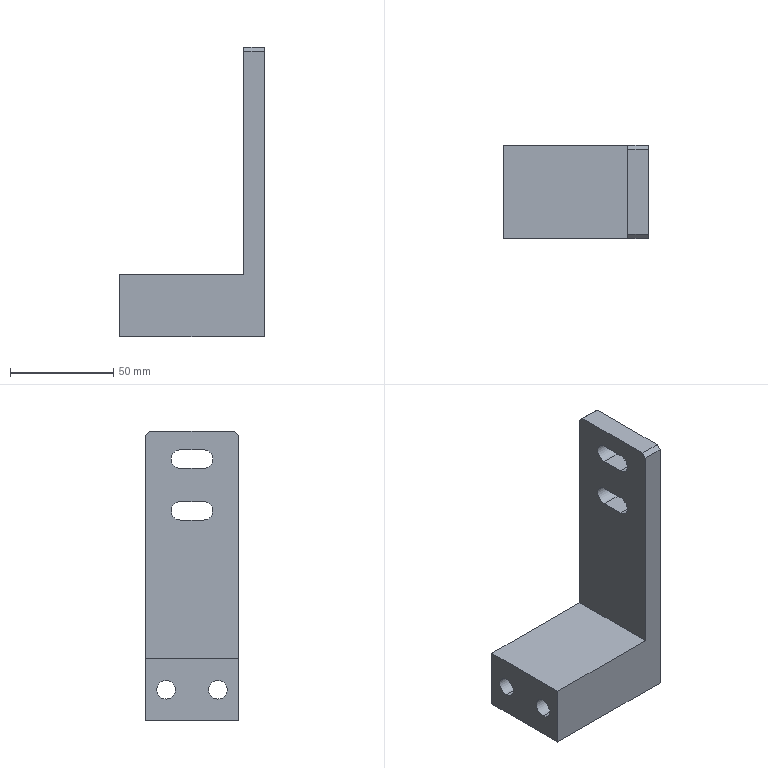Part | SolidWorks | features BaseBody 1 | 1 solid | 28 faces | box 70 x 45 x 140 mm | volume 118230 mm3 | plane 16 | cylinder 12 | commonest cylinder face diameters 9 x8 15 x4
STEP:
#1=CARTESIAN_POINT('',(114.247,1537.,-339.5));
#2=VERTEX_POINT('',#1);
#3=CARTESIAN_POINT('',(114.247,1537.,-354.5));
#4=VERTEX_POINT('',#3);
#5=CARTESIAN_POINT('',(114.247,1537.,-347.));
#6=DIRECTION('',(1.,0.,0.));
#7=DIRECTION('',(0.,0.,-1.));
#8=AXIS2_PLACEMENT_3D('',#5,#6,#7);
#9=CIRCLE('',#8,7.5);
#10=EDGE_CURVE('',#2,#4,#9,.T.);
#11=ORIENTED_EDGE('',*,*,#10,.F.);
#12=CARTESIAN_POINT('',(174.247,1537.,-339.5));
#13=VERTEX_POINT('',#12);
#14=CARTESIAN_POINT('',(174.247,1537.,-339.5));
#15=DIRECTION('',(1.,0.,0.));
#16=VECTOR('',#15,1000.);
#17=LINE('',#14,#16);
#18=EDGE_CURVE('',#2,#13,#17,.T.);
#19=ORIENTED_EDGE('',*,*,#18,.T.);
#20=CARTESIAN_POINT('',(174.247,1537.,-354.5));
#21=VERTEX_POINT('',#20);
#22=CARTESIAN_POINT('',(174.247,1537.,-347.));
#23=DIRECTION('',(1.,0.,0.));
#24=DIRECTION('',(0.,0.,-1.));
#25=AXIS2_PLACEMENT_3D('',#22,#23,#24);
#26=CIRCLE('',#25,7.5);
#27=EDGE_CURVE('',#13,#21,#26,.T.);
#28=ORIENTED_EDGE('',*,*,#27,.T.);
#29=CARTESIAN_POINT('',(174.247,1537.,-354.5));
#30=DIRECTION('',(1.,0.,0.));
#31=VECTOR('',#30,1000.);
#32=LINE('',#29,#31);
#33=EDGE_CURVE('',#4,#21,#32,.T.);
#34=ORIENTED_EDGE('',*,*,#33,.F.);
#35=EDGE_LOOP('',(#11,#19,#28,#34));
#36=FACE_OUTER_BOUND('',#35,.T.);
#37=CARTESIAN_POINT('',(174.247,1537.,-347.));
#38=DIRECTION('',(1.,0.,0.));
#39=DIRECTION('',(0.,0.,-1.));
#40=AXIS2_PLACEMENT_3D('',#37,#38,#39);
#41=CYLINDRICAL_SURFACE('',#40,7.5);
#42=ADVANCED_FACE('',(#36),#41,.F.);
#43=CARTESIAN_POINT('',(114.247,1562.,-339.5));
#44=VERTEX_POINT('',#43);
#45=CARTESIAN_POINT('',(114.247,1562.,-354.5));
#46=VERTEX_POINT('',#45);
#47=CARTESIAN_POINT('',(114.247,1562.,-347.));
#48=DIRECTION('',(1.,0.,0.));
#49=DIRECTION('',(0.,0.,-1.));
#50=AXIS2_PLACEMENT_3D('',#47,#48,#49);
#51=CIRCLE('',#50,7.5);
#52=EDGE_CURVE('',#44,#46,#51,.T.);
#53=ORIENTED_EDGE('',*,*,#52,.F.);
#54=CARTESIAN_POINT('',(174.247,1562.,-339.5));
#55=VERTEX_POINT('',#54);
#56=CARTESIAN_POINT('',(174.247,1562.,-339.5));
#57=DIRECTION('',(1.,0.,0.));
#58=VECTOR('',#57,1000.);
#59=LINE('',#56,#58);
#60=EDGE_CURVE('',#44,#55,#59,.T.);
#61=ORIENTED_EDGE('',*,*,#60,.T.);
#62=CARTESIAN_POINT('',(174.247,1562.,-354.5));
#63=VERTEX_POINT('',#62);
#64=CARTESIAN_POINT('',(174.247,1562.,-347.));
#65=DIRECTION('',(1.,0.,0.));
#66=DIRECTION('',(0.,0.,-1.));
#67=AXIS2_PLACEMENT_3D('',#64,#65,#66);
#68=CIRCLE('',#67,7.5);
#69=EDGE_CURVE('',#55,#63,#68,.T.);
#70=ORIENTED_EDGE('',*,*,#69,.T.);
#71=CARTESIAN_POINT('',(174.247,1562.,-354.5));
#72=DIRECTION('',(1.,0.,0.));
#73=VECTOR('',#72,1000.);
#74=LINE('',#71,#73);
#75=EDGE_CURVE('',#46,#63,#74,.T.);
#76=ORIENTED_EDGE('',*,*,#75,.F.);
#77=EDGE_LOOP('',(#53,#61,#70,#76));
#78=FACE_OUTER_BOUND('',#77,.T.);
#79=CARTESIAN_POINT('',(174.247,1562.,-347.));
#80=DIRECTION('',(1.,0.,0.));
#81=DIRECTION('',(0.,0.,-1.));
#82=AXIS2_PLACEMENT_3D('',#79,#80,#81);
#83=CYLINDRICAL_SURFACE('',#82,7.5);
#84=ADVANCED_FACE('',(#78),#83,.F.);
#85=CARTESIAN_POINT('',(104.247,1537.,-351.5));
#86=VERTEX_POINT('',#85);
#87=CARTESIAN_POINT('',(104.247,1537.,-342.5));
#88=VERTEX_POINT('',#87);
#89=CARTESIAN_POINT('',(104.247,1537.,-347.));
#90=DIRECTION('',(-1.,0.,0.));
#91=DIRECTION('',(0.,0.,-1.));
#92=AXIS2_PLACEMENT_3D('',#89,#90,#91);
#93=CIRCLE('',#92,4.5);
#94=EDGE_CURVE('',#86,#88,#93,.T.);
#95=ORIENTED_EDGE('',*,*,#94,.T.);
#96=CARTESIAN_POINT('',(114.247,1537.,-342.5));
#97=VERTEX_POINT('',#96);
#98=CARTESIAN_POINT('',(174.247,1537.,-342.5));
#99=DIRECTION('',(1.,0.,0.));
#100=VECTOR('',#99,1000.);
#101=LINE('',#98,#100);
#102=EDGE_CURVE('',#88,#97,#101,.T.);
#103=ORIENTED_EDGE('',*,*,#102,.T.);
#104=CARTESIAN_POINT('',(114.247,1537.,-351.5));
#105=VERTEX_POINT('',#104);
#106=CARTESIAN_POINT('',(114.247,1537.,-347.));
#107=DIRECTION('',(1.,0.,0.));
#108=DIRECTION('',(0.,0.,-1.));
#109=AXIS2_PLACEMENT_3D('',#106,#107,#108);
#110=CIRCLE('',#109,4.5);
#111=EDGE_CURVE('',#97,#105,#110,.T.);
#112=ORIENTED_EDGE('',*,*,#111,.T.);
#113=CARTESIAN_POINT('',(174.247,1537.,-351.5));
#114=DIRECTION('',(1.,0.,0.));
#115=VECTOR('',#114,1000.);
#116=LINE('',#113,#115);
#117=EDGE_CURVE('',#86,#105,#116,.T.);
#118=ORIENTED_EDGE('',*,*,#117,.F.);
#119=EDGE_LOOP('',(#95,#103,#112,#118));
#120=FACE_OUTER_BOUND('',#119,.T.);
#121=CARTESIAN_POINT('',(174.247,1537.,-347.));
#122=DIRECTION('',(1.,0.,0.));
#123=DIRECTION('',(0.,0.,-1.));
#124=AXIS2_PLACEMENT_3D('',#121,#122,#123);
#125=CYLINDRICAL_SURFACE('',#124,4.5);
#126=ADVANCED_FACE('',(#120),#125,.F.);
#127=CARTESIAN_POINT('',(104.247,1562.,-351.5));
#128=VERTEX_POINT('',#127);
#129=CARTESIAN_POINT('',(104.247,1562.,-342.5));
#130=VERTEX_POINT('',#129);
#131=CARTESIAN_POINT('',(104.247,1562.,-347.));
#132=DIRECTION('',(-1.,0.,0.));
#133=DIRECTION('',(0.,0.,-1.));
#134=AXIS2_PLACEMENT_3D('',#131,#132,#133);
#135=CIRCLE('',#134,4.5);
#136=EDGE_CURVE('',#128,#130,#135,.T.);
#137=ORIENTED_EDGE('',*,*,#136,.T.);
#138=CARTESIAN_POINT('',(114.247,1562.,-342.5));
#139=VERTEX_POINT('',#138);
#140=CARTESIAN_POINT('',(174.247,1562.,-342.5));
#141=DIRECTION('',(1.,0.,0.));
#142=VECTOR('',#141,1000.);
#143=LINE('',#140,#142);
#144=EDGE_CURVE('',#130,#139,#143,.T.);
#145=ORIENTED_EDGE('',*,*,#144,.T.);
#146=CARTESIAN_POINT('',(114.247,1562.,-351.5));
#147=VERTEX_POINT('',#146);
#148=CARTESIAN_POINT('',(114.247,1562.,-347.));
#149=DIRECTION('',(1.,0.,0.));
#150=DIRECTION('',(0.,0.,-1.));
#151=AXIS2_PLACEMENT_3D('',#148,#149,#150);
#152=CIRCLE('',#151,4.5);
#153=EDGE_CURVE('',#139,#147,#152,.T.);
#154=ORIENTED_EDGE('',*,*,#153,.T.);
#155=CARTESIAN_POINT('',(174.247,1562.,-351.5));
#156=DIRECTION('',(1.,0.,0.));
#157=VECTOR('',#156,1000.);
#158=LINE('',#155,#157);
#159=EDGE_CURVE('',#128,#147,#158,.T.);
#160=ORIENTED_EDGE('',*,*,#159,.F.);
#161=EDGE_LOOP('',(#137,#145,#154,#160));
#162=FACE_OUTER_BOUND('',#161,.T.);
#163=CARTESIAN_POINT('',(174.247,1562.,-347.));
#164=DIRECTION('',(1.,0.,0.));
#165=DIRECTION('',(0.,0.,-1.));
#166=AXIS2_PLACEMENT_3D('',#163,#164,#165);
#167=CYLINDRICAL_SURFACE('',#166,4.5);
#168=ADVANCED_FACE('',(#162),#167,.F.);
#169=CARTESIAN_POINT('',(174.247,1544.,-240.));
#170=VERTEX_POINT('',#169);
#171=CARTESIAN_POINT('',(174.247,1555.,-240.));
#172=VERTEX_POINT('',#171);
#173=CARTESIAN_POINT('',(174.247,1549.5,-240.));
#174=DIRECTION('',(0.,1.,0.));
#175=VECTOR('',#174,1000.);
#176=LINE('',#173,#175);
#177=EDGE_CURVE('',#170,#172,#176,.T.);
#178=ORIENTED_EDGE('',*,*,#177,.F.);
#179=CARTESIAN_POINT('',(174.247,1544.,-231.));
#180=VERTEX_POINT('',#179);
#181=CARTESIAN_POINT('',(174.247,1544.,-235.5));
#182=DIRECTION('',(1.,0.,0.));
#183=DIRECTION('',(0.,0.,-1.));
#184=AXIS2_PLACEMENT_3D('',#181,#182,#183);
#185=CIRCLE('',#184,4.5);
#186=EDGE_CURVE('',#180,#170,#185,.T.);
#187=ORIENTED_EDGE('',*,*,#186,.F.);
#188=CARTESIAN_POINT('',(174.247,1555.,-231.));
#189=VERTEX_POINT('',#188);
#190=CARTESIAN_POINT('',(174.247,1549.5,-231.));
#191=DIRECTION('',(0.,-1.,0.));
#192=VECTOR('',#191,1000.);
#193=LINE('',#190,#192);
#194=EDGE_CURVE('',#189,#180,#193,.T.);
#195=ORIENTED_EDGE('',*,*,#194,.F.);
#196=CARTESIAN_POINT('',(174.247,1555.,-235.5));
#197=DIRECTION('',(1.,0.,0.));
#198=DIRECTION('',(0.,0.,-1.));
#199=AXIS2_PLACEMENT_3D('',#196,#197,#198);
#200=CIRCLE('',#199,4.5);
#201=EDGE_CURVE('',#172,#189,#200,.T.);
#202=ORIENTED_EDGE('',*,*,#201,.F.);
#203=EDGE_LOOP('',(#178,#187,#195,#202));
#204=FACE_BOUND('',#203,.T.);
#205=CARTESIAN_POINT('',(174.247,1555.,-256.));
#206=VERTEX_POINT('',#205);
#207=CARTESIAN_POINT('',(174.247,1544.,-256.));
#208=VERTEX_POINT('',#207);
#209=CARTESIAN_POINT('',(174.247,1549.5,-256.));
#210=DIRECTION('',(0.,-1.,0.));
#211=VECTOR('',#210,1000.);
#212=LINE('',#209,#211);
#213=EDGE_CURVE('',#206,#208,#212,.T.);
#214=ORIENTED_EDGE('',*,*,#213,.F.);
#215=CARTESIAN_POINT('',(174.247,1555.,-265.));
#216=VERTEX_POINT('',#215);
#217=CARTESIAN_POINT('',(174.247,1555.,-260.5));
#218=DIRECTION('',(1.,0.,0.));
#219=DIRECTION('',(0.,0.,-1.));
#220=AXIS2_PLACEMENT_3D('',#217,#218,#219);
#221=CIRCLE('',#220,4.5);
#222=EDGE_CURVE('',#216,#206,#221,.T.);
#223=ORIENTED_EDGE('',*,*,#222,.F.);
#224=CARTESIAN_POINT('',(174.247,1544.,-265.));
#225=VERTEX_POINT('',#224);
#226=CARTESIAN_POINT('',(174.247,1549.5,-265.));
#227=DIRECTION('',(0.,1.,0.));
#228=VECTOR('',#227,1000.);
#229=LINE('',#226,#228);
#230=EDGE_CURVE('',#225,#216,#229,.T.);
#231=ORIENTED_EDGE('',*,*,#230,.F.);
#232=CARTESIAN_POINT('',(174.247,1544.,-260.5));
#233=DIRECTION('',(1.,0.,0.));
#234=DIRECTION('',(0.,0.,-1.));
#235=AXIS2_PLACEMENT_3D('',#232,#233,#234);
#236=CIRCLE('',#235,4.5);
#237=EDGE_CURVE('',#208,#225,#236,.T.);
#238=ORIENTED_EDGE('',*,*,#237,.F.);
#239=EDGE_LOOP('',(#214,#223,#231,#238));
#240=FACE_BOUND('',#239,.T.);
#241=CARTESIAN_POINT('',(174.247,1537.,-347.));
#242=DIRECTION('',(1.,0.,0.));
#243=DIRECTION('',(0.,0.,-1.));
#244=AXIS2_PLACEMENT_3D('',#241,#242,#243);
#245=CIRCLE('',#244,7.5);
#246=EDGE_CURVE('',#21,#13,#245,.T.);
#247=ORIENTED_EDGE('',*,*,#246,.F.);
#248=ORIENTED_EDGE('',*,*,#27,.F.);
#249=EDGE_LOOP('',(#247,#248));
#250=FACE_BOUND('',#249,.T.);
#251=CARTESIAN_POINT('',(174.247,1562.,-347.));
#252=DIRECTION('',(1.,0.,0.));
#253=DIRECTION('',(0.,0.,-1.));
#254=AXIS2_PLACEMENT_3D('',#251,#252,#253);
#255=CIRCLE('',#254,7.5);
#256=EDGE_CURVE('',#63,#55,#255,.T.);
#257=ORIENTED_EDGE('',*,*,#256,.F.);
#258=ORIENTED_EDGE('',*,*,#69,.F.);
#259=EDGE_LOOP('',(#257,#258));
#260=FACE_BOUND('',#259,.T.);
#261=CARTESIAN_POINT('',(174.247,1529.,-222.));
#262=VERTEX_POINT('',#261);
#263=CARTESIAN_POINT('',(174.247,1570.,-222.));
#264=VERTEX_POINT('',#263);
#265=CARTESIAN_POINT('',(174.247,1549.5,-222.));
#266=DIRECTION('',(0.,1.,0.));
#267=VECTOR('',#266,1000.);
#268=LINE('',#265,#267);
#269=EDGE_CURVE('',#262,#264,#268,.T.);
#270=ORIENTED_EDGE('',*,*,#269,.F.);
#271=CARTESIAN_POINT('',(174.247,1527.,-224.));
#272=VERTEX_POINT('',#271);
#273=CARTESIAN_POINT('',(174.247,1527.,-224.));
#274=DIRECTION('',(0.,0.7071,0.7071));
#275=VECTOR('',#274,1000.);
#276=LINE('',#273,#275);
#277=EDGE_CURVE('',#272,#262,#276,.T.);
#278=ORIENTED_EDGE('',*,*,#277,.F.);
#279=CARTESIAN_POINT('',(174.247,1527.,-362.));
#280=VERTEX_POINT('',#279);
#281=CARTESIAN_POINT('',(174.247,1527.,-292.));
#282=DIRECTION('',(0.,0.,1.));
#283=VECTOR('',#282,1000.);
#284=LINE('',#281,#283);
#285=EDGE_CURVE('',#280,#272,#284,.T.);
#286=ORIENTED_EDGE('',*,*,#285,.F.);
#287=CARTESIAN_POINT('',(174.247,1572.,-362.));
#288=VERTEX_POINT('',#287);
#289=CARTESIAN_POINT('',(174.247,1549.5,-362.));
#290=DIRECTION('',(0.,-1.,0.));
#291=VECTOR('',#290,1000.);
#292=LINE('',#289,#291);
#293=EDGE_CURVE('',#288,#280,#292,.T.);
#294=ORIENTED_EDGE('',*,*,#293,.F.);
#295=CARTESIAN_POINT('',(174.247,1572.,-224.));
#296=VERTEX_POINT('',#295);
#297=CARTESIAN_POINT('',(174.247,1572.,-292.));
#298=DIRECTION('',(0.,0.,-1.));
#299=VECTOR('',#298,1000.);
#300=LINE('',#297,#299);
#301=EDGE_CURVE('',#296,#288,#300,.T.);
#302=ORIENTED_EDGE('',*,*,#301,.F.);
#303=CARTESIAN_POINT('',(174.247,1570.,-222.));
#304=DIRECTION('',(0.,0.7071,-0.7071));
#305=VECTOR('',#304,1000.);
#306=LINE('',#303,#305);
#307=EDGE_CURVE('',#264,#296,#306,.T.);
#308=ORIENTED_EDGE('',*,*,#307,.F.);
#309=EDGE_LOOP('',(#270,#278,#286,#294,#302,#308));
#310=FACE_OUTER_BOUND('',#309,.T.);
#311=CARTESIAN_POINT('',(174.247,1549.5,-292.));
#312=DIRECTION('',(-1.,0.,0.));
#313=DIRECTION('',(0.,0.,1.));
#314=AXIS2_PLACEMENT_3D('',#311,#312,#313);
#315=PLANE('',#314);
#316=ADVANCED_FACE('',(#204,#240,#250,#260,#310),#315,.F.);
#317=ORIENTED_EDGE('',*,*,#177,.T.);
#318=CARTESIAN_POINT('',(164.247,1555.,-240.));
#319=VERTEX_POINT('',#318);
#320=CARTESIAN_POINT('',(174.247,1555.,-240.));
#321=DIRECTION('',(1.,0.,0.));
#322=VECTOR('',#321,1000.);
#323=LINE('',#320,#322);
#324=EDGE_CURVE('',#319,#172,#323,.T.);
#325=ORIENTED_EDGE('',*,*,#324,.F.);
#326=CARTESIAN_POINT('',(164.247,1544.,-240.));
#327=VERTEX_POINT('',#326);
#328=CARTESIAN_POINT('',(164.247,1544.,-240.));
#329=DIRECTION('',(0.,1.,0.));
#330=VECTOR('',#329,1000.);
#331=LINE('',#328,#330);
#332=EDGE_CURVE('',#327,#319,#331,.T.);
#333=ORIENTED_EDGE('',*,*,#332,.F.);
#334=CARTESIAN_POINT('',(174.247,1544.,-240.));
#335=DIRECTION('',(-1.,0.,0.));
#336=VECTOR('',#335,1000.);
#337=LINE('',#334,#336);
#338=EDGE_CURVE('',#170,#327,#337,.T.);
#339=ORIENTED_EDGE('',*,*,#338,.F.);
#340=EDGE_LOOP('',(#317,#325,#333,#339));
#341=FACE_OUTER_BOUND('',#340,.T.);
#342=CARTESIAN_POINT('',(174.247,1544.,-240.));
#343=DIRECTION('',(0.,0.,-1.));
#344=DIRECTION('',(-1.,0.,0.));
#345=AXIS2_PLACEMENT_3D('',#342,#343,#344);
#346=PLANE('',#345);
#347=ADVANCED_FACE('',(#341),#346,.F.);
#348=ORIENTED_EDGE('',*,*,#186,.T.);
#349=ORIENTED_EDGE('',*,*,#338,.T.);
#350=CARTESIAN_POINT('',(164.247,1544.,-231.));
#351=VERTEX_POINT('',#350);
#352=CARTESIAN_POINT('',(164.247,1544.,-235.5));
#353=DIRECTION('',(1.,0.,0.));
#354=DIRECTION('',(0.,0.,-1.));
#355=AXIS2_PLACEMENT_3D('',#352,#353,#354);
#356=CIRCLE('',#355,4.5);
#357=EDGE_CURVE('',#351,#327,#356,.T.);
#358=ORIENTED_EDGE('',*,*,#357,.F.);
#359=CARTESIAN_POINT('',(174.247,1544.,-231.));
#360=DIRECTION('',(-1.,0.,0.));
#361=VECTOR('',#360,1000.);
#362=LINE('',#359,#361);
#363=EDGE_CURVE('',#180,#351,#362,.T.);
#364=ORIENTED_EDGE('',*,*,#363,.F.);
#365=EDGE_LOOP('',(#348,#349,#358,#364));
#366=FACE_OUTER_BOUND('',#365,.T.);
#367=CARTESIAN_POINT('',(174.247,1544.,-235.5));
#368=DIRECTION('',(1.,0.,0.));
#369=DIRECTION('',(0.,0.,-1.));
#370=AXIS2_PLACEMENT_3D('',#367,#368,#369);
#371=CYLINDRICAL_SURFACE('',#370,4.5);
#372=ADVANCED_FACE('',(#366),#371,.F.);
#373=CARTESIAN_POINT('',(164.247,1555.,-231.));
#374=VERTEX_POINT('',#373);
#375=CARTESIAN_POINT('',(164.247,1544.,-231.));
#376=DIRECTION('',(0.,1.,0.));
#377=VECTOR('',#376,1000.);
#378=LINE('',#375,#377);
#379=EDGE_CURVE('',#351,#374,#378,.T.);
#380=ORIENTED_EDGE('',*,*,#379,.T.);
#381=CARTESIAN_POINT('',(104.247,1555.,-231.));
#382=DIRECTION('',(1.,0.,0.));
#383=VECTOR('',#382,1000.);
#384=LINE('',#381,#383);
#385=EDGE_CURVE('',#374,#189,#384,.T.);
#386=ORIENTED_EDGE('',*,*,#385,.T.);
#387=ORIENTED_EDGE('',*,*,#194,.T.);
#388=ORIENTED_EDGE('',*,*,#363,.T.);
#389=EDGE_LOOP('',(#380,#386,#387,#388));
#390=FACE_OUTER_BOUND('',#389,.T.);
#391=CARTESIAN_POINT('',(104.247,1544.,-231.));
#392=DIRECTION('',(0.,0.,-1.));
#393=DIRECTION('',(-1.,0.,0.));
#394=AXIS2_PLACEMENT_3D('',#391,#392,#393);
#395=PLANE('',#394);
#396=ADVANCED_FACE('',(#390),#395,.T.);
#397=ORIENTED_EDGE('',*,*,#324,.T.);
#398=ORIENTED_EDGE('',*,*,#201,.T.);
#399=ORIENTED_EDGE('',*,*,#385,.F.);
#400=CARTESIAN_POINT('',(164.247,1555.,-235.5));
#401=DIRECTION('',(1.,0.,0.));
#402=DIRECTION('',(0.,0.,-1.));
#403=AXIS2_PLACEMENT_3D('',#400,#401,#402);
#404=CIRCLE('',#403,4.5);
#405=EDGE_CURVE('',#319,#374,#404,.T.);
#406=ORIENTED_EDGE('',*,*,#405,.F.);
#407=EDGE_LOOP('',(#397,#398,#399,#406));
#408=FACE_OUTER_BOUND('',#407,.T.);
#409=CARTESIAN_POINT('',(174.247,1555.,-235.5));
#410=DIRECTION('',(1.,0.,0.));
#411=DIRECTION('',(0.,0.,-1.));
#412=AXIS2_PLACEMENT_3D('',#409,#410,#411);
#413=CYLINDRICAL_SURFACE('',#412,4.5);
#414=ADVANCED_FACE('',(#408),#413,.F.);
#415=CARTESIAN_POINT('',(164.247,1544.,-256.));
#416=VERTEX_POINT('',#415);
#417=CARTESIAN_POINT('',(174.247,1544.,-256.));
#418=DIRECTION('',(-1.,0.,0.));
#419=VECTOR('',#418,1000.);
#420=LINE('',#417,#419);
#421=EDGE_CURVE('',#208,#416,#420,.T.);
#422=ORIENTED_EDGE('',*,*,#421,.F.);
#423=ORIENTED_EDGE('',*,*,#237,.T.);
#424=CARTESIAN_POINT('',(164.247,1544.,-265.));
#425=VERTEX_POINT('',#424);
#426=CARTESIAN_POINT('',(174.247,1544.,-265.));
#427=DIRECTION('',(1.,0.,0.));
#428=VECTOR('',#427,1000.);
#429=LINE('',#426,#428);
#430=EDGE_CURVE('',#425,#225,#429,.T.);
#431=ORIENTED_EDGE('',*,*,#430,.F.);
#432=CARTESIAN_POINT('',(164.247,1544.,-260.5));
#433=DIRECTION('',(1.,0.,0.));
#434=DIRECTION('',(0.,0.,-1.));
#435=AXIS2_PLACEMENT_3D('',#432,#433,#434);
#436=CIRCLE('',#435,4.5);
#437=EDGE_CURVE('',#416,#425,#436,.T.);
#438=ORIENTED_EDGE('',*,*,#437,.F.);
#439=EDGE_LOOP('',(#422,#423,#431,#438));
#440=FACE_OUTER_BOUND('',#439,.T.);
#441=CARTESIAN_POINT('',(174.247,1544.,-260.5));
#442=DIRECTION('',(1.,0.,0.));
#443=DIRECTION('',(0.,0.,-1.));
#444=AXIS2_PLACEMENT_3D('',#441,#442,#443);
#445=CYLINDRICAL_SURFACE('',#444,4.5);
#446=ADVANCED_FACE('',(#440),#445,.F.);
#447=CARTESIAN_POINT('',(164.247,1555.,-256.));
#448=VERTEX_POINT('',#447);
#449=CARTESIAN_POINT('',(164.247,1544.,-256.));
#450=DIRECTION('',(0.,1.,0.));
#451=VECTOR('',#450,1000.);
#452=LINE('',#449,#451);
#453=EDGE_CURVE('',#416,#448,#452,.T.);
#454=ORIENTED_EDGE('',*,*,#453,.T.);
#455=CARTESIAN_POINT('',(104.247,1555.,-256.));
#456=DIRECTION('',(1.,0.,0.));
#457=VECTOR('',#456,1000.);
#458=LINE('',#455,#457);
#459=EDGE_CURVE('',#448,#206,#458,.T.);
#460=ORIENTED_EDGE('',*,*,#459,.T.);
#461=ORIENTED_EDGE('',*,*,#213,.T.);
#462=ORIENTED_EDGE('',*,*,#421,.T.);
#463=EDGE_LOOP('',(#454,#460,#461,#462));
#464=FACE_OUTER_BOUND('',#463,.T.);
#465=CARTESIAN_POINT('',(104.247,1544.,-256.));
#466=DIRECTION('',(0.,0.,-1.));
#467=DIRECTION('',(-1.,0.,0.));
#468=AXIS2_PLACEMENT_3D('',#465,#466,#467);
#469=PLANE('',#468);
#470=ADVANCED_FACE('',(#464),#469,.T.);
#471=CARTESIAN_POINT('',(164.247,1555.,-265.));
#472=VERTEX_POINT('',#471);
#473=CARTESIAN_POINT('',(174.247,1555.,-265.));
#474=DIRECTION('',(-1.,0.,0.));
#475=VECTOR('',#474,1000.);
#476=LINE('',#473,#475);
#477=EDGE_CURVE('',#216,#472,#476,.T.);
#478=ORIENTED_EDGE('',*,*,#477,.F.);
#479=ORIENTED_EDGE('',*,*,#222,.T.);
#480=ORIENTED_EDGE('',*,*,#459,.F.);
#481=CARTESIAN_POINT('',(164.247,1555.,-260.5));
#482=DIRECTION('',(1.,0.,0.));
#483=DIRECTION('',(0.,0.,-1.));
#484=AXIS2_PLACEMENT_3D('',#481,#482,#483);
#485=CIRCLE('',#484,4.5);
#486=EDGE_CURVE('',#472,#448,#485,.T.);
#487=ORIENTED_EDGE('',*,*,#486,.F.);
#488=EDGE_LOOP('',(#478,#479,#480,#487));
#489=FACE_OUTER_BOUND('',#488,.T.);
#490=CARTESIAN_POINT('',(174.247,1555.,-260.5));
#491=DIRECTION('',(1.,0.,0.));
#492=DIRECTION('',(0.,0.,-1.));
#493=AXIS2_PLACEMENT_3D('',#490,#491,#492);
#494=CYLINDRICAL_SURFACE('',#493,4.5);
#495=ADVANCED_FACE('',(#489),#494,.F.);
#496=ORIENTED_EDGE('',*,*,#230,.T.);
#497=ORIENTED_EDGE('',*,*,#477,.T.);
#498=CARTESIAN_POINT('',(164.247,1544.,-265.));
#499=DIRECTION('',(0.,1.,0.));
#500=VECTOR('',#499,1000.);
#501=LINE('',#498,#500);
#502=EDGE_CURVE('',#425,#472,#501,.T.);
#503=ORIENTED_EDGE('',*,*,#502,.F.);
#504=ORIENTED_EDGE('',*,*,#430,.T.);
#505=EDGE_LOOP('',(#496,#497,#503,#504));
#506=FACE_OUTER_BOUND('',#505,.T.);
#507=CARTESIAN_POINT('',(174.247,1544.,-265.));
#508=DIRECTION('',(0.,0.,-1.));
#509=DIRECTION('',(-1.,0.,0.));
#510=AXIS2_PLACEMENT_3D('',#507,#508,#509);
#511=PLANE('',#510);
#512=ADVANCED_FACE('',(#506),#511,.F.);
#513=ORIENTED_EDGE('',*,*,#18,.F.);
#514=CARTESIAN_POINT('',(114.247,1537.,-347.));
#515=DIRECTION('',(1.,0.,0.));
#516=DIRECTION('',(0.,0.,-1.));
#517=AXIS2_PLACEMENT_3D('',#514,#515,#516);
#518=CIRCLE('',#517,7.5);
#519=EDGE_CURVE('',#4,#2,#518,.T.);
#520=ORIENTED_EDGE('',*,*,#519,.F.);
#521=ORIENTED_EDGE('',*,*,#33,.T.);
#522=ORIENTED_EDGE('',*,*,#246,.T.);
#523=EDGE_LOOP('',(#513,#520,#521,#522));
#524=FACE_OUTER_BOUND('',#523,.T.);
#525=CARTESIAN_POINT('',(174.247,1537.,-347.));
#526=DIRECTION('',(1.,0.,0.));
#527=DIRECTION('',(0.,0.,-1.));
#528=AXIS2_PLACEMENT_3D('',#525,#526,#527);
#529=CYLINDRICAL_SURFACE('',#528,7.5);
#530=ADVANCED_FACE('',(#524),#529,.F.);
#531=ORIENTED_EDGE('',*,*,#60,.F.);
#532=CARTESIAN_POINT('',(114.247,1562.,-347.));
#533=DIRECTION('',(1.,0.,0.));
#534=DIRECTION('',(0.,0.,-1.));
#535=AXIS2_PLACEMENT_3D('',#532,#533,#534);
#536=CIRCLE('',#535,7.5);
#537=EDGE_CURVE('',#46,#44,#536,.T.);
#538=ORIENTED_EDGE('',*,*,#537,.F.);
#539=ORIENTED_EDGE('',*,*,#75,.T.);
#540=ORIENTED_EDGE('',*,*,#256,.T.);
#541=EDGE_LOOP('',(#531,#538,#539,#540));
#542=FACE_OUTER_BOUND('',#541,.T.);
#543=CARTESIAN_POINT('',(174.247,1562.,-347.));
#544=DIRECTION('',(1.,0.,0.));
#545=DIRECTION('',(0.,0.,-1.));
#546=AXIS2_PLACEMENT_3D('',#543,#544,#545);
#547=CYLINDRICAL_SURFACE('',#546,7.5);
#548=ADVANCED_FACE('',(#542),#547,.F.);
#549=ORIENTED_EDGE('',*,*,#307,.T.);
#550=CARTESIAN_POINT('',(164.247,1572.,-224.));
#551=VERTEX_POINT('',#550);
#552=CARTESIAN_POINT('',(164.247,1572.,-224.));
#553=DIRECTION('',(1.,0.,0.));
#554=VECTOR('',#553,1000.);
#555=LINE('',#552,#554);
#556=EDGE_CURVE('',#551,#296,#555,.T.);
#557=ORIENTED_EDGE('',*,*,#556,.F.);
#558=CARTESIAN_POINT('',(164.247,1570.,-222.));
#559=VERTEX_POINT('',#558);
#560=CARTESIAN_POINT('',(164.247,1572.,-224.));
#561=DIRECTION('',(0.,0.7071,-0.7071));
#562=VECTOR('',#561,1000.);
#563=LINE('',#560,#562);
#564=EDGE_CURVE('',#559,#551,#563,.T.);
#565=ORIENTED_EDGE('',*,*,#564,.F.);
#566=CARTESIAN_POINT('',(164.247,1570.,-222.));
#567=DIRECTION('',(-1.,0.,0.));
#568=VECTOR('',#567,1000.);
#569=LINE('',#566,#568);
#570=EDGE_CURVE('',#264,#559,#569,.T.);
#571=ORIENTED_EDGE('',*,*,#570,.F.);
#572=EDGE_LOOP('',(#549,#557,#565,#571));
#573=FACE_OUTER_BOUND('',#572,.T.);
#574=CARTESIAN_POINT('',(164.247,1572.,-224.));
#575=DIRECTION('',(0.,-0.7071,-0.7071));
#576=DIRECTION('',(0.,0.7071,-0.7071));
#577=AXIS2_PLACEMENT_3D('',#574,#575,#576);
#578=PLANE('',#577);
#579=ADVANCED_FACE('',(#573),#578,.F.);
#580=CARTESIAN_POINT('',(164.247,1529.,-222.));
#581=VERTEX_POINT('',#580);
#582=CARTESIAN_POINT('',(164.247,1572.,-222.));
#583=DIRECTION('',(0.,1.,0.));
#584=VECTOR('',#583,1000.);
#585=LINE('',#582,#584);
#586=EDGE_CURVE('',#581,#559,#585,.T.);
#587=ORIENTED_EDGE('',*,*,#586,.F.);
#588=CARTESIAN_POINT('',(164.247,1529.,-222.));
#589=DIRECTION('',(-1.,0.,0.));
#590=VECTOR('',#589,1000.);
#591=LINE('',#588,#590);
#592=EDGE_CURVE('',#262,#581,#591,.T.);
#593=ORIENTED_EDGE('',*,*,#592,.F.);
#594=ORIENTED_EDGE('',*,*,#269,.T.);
#595=ORIENTED_EDGE('',*,*,#570,.T.);
#596=EDGE_LOOP('',(#587,#593,#594,#595));
#597=FACE_OUTER_BOUND('',#596,.T.);
#598=CARTESIAN_POINT('',(164.247,1572.,-222.));
#599=DIRECTION('',(0.,0.,-1.));
#600=DIRECTION('',(-1.,0.,0.));
#601=AXIS2_PLACEMENT_3D('',#598,#599,#600);
#602=PLANE('',#601);
#603=ADVANCED_FACE('',(#597),#602,.F.);
#604=ORIENTED_EDGE('',*,*,#277,.T.);
#605=ORIENTED_EDGE('',*,*,#592,.T.);
#606=CARTESIAN_POINT('',(164.247,1527.,-224.));
#607=VERTEX_POINT('',#606);
#608=CARTESIAN_POINT('',(164.247,1529.,-222.));
#609=DIRECTION('',(0.,0.7071,0.7071));
#610=VECTOR('',#609,1000.);
#611=LINE('',#608,#610);
#612=EDGE_CURVE('',#607,#581,#611,.T.);
#613=ORIENTED_EDGE('',*,*,#612,.F.);
#614=CARTESIAN_POINT('',(164.247,1527.,-224.));
#615=DIRECTION('',(-1.,0.,0.));
#616=VECTOR('',#615,1000.);
#617=LINE('',#614,#616);
#618=EDGE_CURVE('',#272,#607,#617,.T.);
#619=ORIENTED_EDGE('',*,*,#618,.F.);
#620=EDGE_LOOP('',(#604,#605,#613,#619));
#621=FACE_OUTER_BOUND('',#620,.T.);
#622=CARTESIAN_POINT('',(164.247,1529.,-222.));
#623=DIRECTION('',(0.,0.7071,-0.7071));
#624=DIRECTION('',(0.,0.7071,0.7071));
#625=AXIS2_PLACEMENT_3D('',#622,#623,#624);
#626=PLANE('',#625);
#627=ADVANCED_FACE('',(#621),#626,.F.);
#628=CARTESIAN_POINT('',(164.247,1527.,-332.));
#629=VERTEX_POINT('',#628);
#630=CARTESIAN_POINT('',(164.247,1527.,-222.));
#631=DIRECTION('',(0.,0.,1.));
#632=VECTOR('',#631,1000.);
#633=LINE('',#630,#632);
#634=EDGE_CURVE('',#629,#607,#633,.T.);
#635=ORIENTED_EDGE('',*,*,#634,.F.);
#636=CARTESIAN_POINT('',(104.247,1527.,-332.));
#637=VERTEX_POINT('',#636);
#638=CARTESIAN_POINT('',(164.247,1527.,-332.));
#639=DIRECTION('',(1.,0.,0.));
#640=VECTOR('',#639,1000.);
#641=LINE('',#638,#640);
#642=EDGE_CURVE('',#637,#629,#641,.T.);
#643=ORIENTED_EDGE('',*,*,#642,.F.);
#644=CARTESIAN_POINT('',(104.247,1527.,-362.));
#645=VERTEX_POINT('',#644);
#646=CARTESIAN_POINT('',(104.247,1527.,-222.));
#647=DIRECTION('',(0.,0.,1.));
#648=VECTOR('',#647,1000.);
#649=LINE('',#646,#648);
#650=EDGE_CURVE('',#645,#637,#649,.T.);
#651=ORIENTED_EDGE('',*,*,#650,.F.);
#652=CARTESIAN_POINT('',(164.247,1527.,-362.));
#653=DIRECTION('',(-1.,0.,0.));
#654=VECTOR('',#653,1000.);
#655=LINE('',#652,#654);
#656=EDGE_CURVE('',#280,#645,#655,.T.);
#657=ORIENTED_EDGE('',*,*,#656,.F.);
#658=ORIENTED_EDGE('',*,*,#285,.T.);
#659=ORIENTED_EDGE('',*,*,#618,.T.);
#660=EDGE_LOOP('',(#635,#643,#651,#657,#658,#659));
#661=FACE_OUTER_BOUND('',#660,.T.);
#662=CARTESIAN_POINT('',(164.247,1527.,-222.));
#663=DIRECTION('',(0.,1.,0.));
#664=DIRECTION('',(0.,0.,1.));
#665=AXIS2_PLACEMENT_3D('',#662,#663,#664);
#666=PLANE('',#665);
#667=ADVANCED_FACE('',(#661),#666,.F.);
#668=CARTESIAN_POINT('',(104.247,1572.,-362.));
#669=VERTEX_POINT('',#668);
#670=CARTESIAN_POINT('',(104.247,1572.,-362.));
#671=DIRECTION('',(0.,-1.,0.));
#672=VECTOR('',#671,1000.);
#673=LINE('',#670,#672);
#674=EDGE_CURVE('',#669,#645,#673,.T.);
#675=ORIENTED_EDGE('',*,*,#674,.F.);
#676=CARTESIAN_POINT('',(164.247,1572.,-362.));
#677=DIRECTION('',(-1.,0.,0.));
#678=VECTOR('',#677,1000.);
#679=LINE('',#676,#678);
#680=EDGE_CURVE('',#288,#669,#679,.T.);
#681=ORIENTED_EDGE('',*,*,#680,.F.);
#682=ORIENTED_EDGE('',*,*,#293,.T.);
#683=ORIENTED_EDGE('',*,*,#656,.T.);
#684=EDGE_LOOP('',(#675,#681,#682,#683));
#685=FACE_OUTER_BOUND('',#684,.T.);
#686=CARTESIAN_POINT('',(164.247,1572.,-362.));
#687=DIRECTION('',(0.,0.,1.));
#688=DIRECTION('',(1.,0.,0.));
#689=AXIS2_PLACEMENT_3D('',#686,#687,#688);
#690=PLANE('',#689);
#691=ADVANCED_FACE('',(#685),#690,.F.);
#692=ORIENTED_EDGE('',*,*,#301,.T.);
#693=ORIENTED_EDGE('',*,*,#680,.T.);
#694=CARTESIAN_POINT('',(104.247,1572.,-332.));
#695=VERTEX_POINT('',#694);
#696=CARTESIAN_POINT('',(104.247,1572.,-222.));
#697=DIRECTION('',(0.,0.,-1.));
#698=VECTOR('',#697,1000.);
#699=LINE('',#696,#698);
#700=EDGE_CURVE('',#695,#669,#699,.T.);
#701=ORIENTED_EDGE('',*,*,#700,.F.);
#702=CARTESIAN_POINT('',(164.247,1572.,-332.));
#703=VERTEX_POINT('',#702);
#704=CARTESIAN_POINT('',(164.247,1572.,-332.));
#705=DIRECTION('',(-1.,0.,0.));
#706=VECTOR('',#705,1000.);
#707=LINE('',#704,#706);
#708=EDGE_CURVE('',#703,#695,#707,.T.);
#709=ORIENTED_EDGE('',*,*,#708,.F.);
#710=CARTESIAN_POINT('',(164.247,1572.,-222.));
#711=DIRECTION('',(0.,0.,-1.));
#712=VECTOR('',#711,1000.);
#713=LINE('',#710,#712);
#714=EDGE_CURVE('',#551,#703,#713,.T.);
#715=ORIENTED_EDGE('',*,*,#714,.F.);
#716=ORIENTED_EDGE('',*,*,#556,.T.);
#717=EDGE_LOOP('',(#692,#693,#701,#709,#715,#716));
#718=FACE_OUTER_BOUND('',#717,.T.);
#719=CARTESIAN_POINT('',(164.247,1572.,-222.));
#720=DIRECTION('',(0.,-1.,0.));
#721=DIRECTION('',(0.,0.,-1.));
#722=AXIS2_PLACEMENT_3D('',#719,#720,#721);
#723=PLANE('',#722);
#724=ADVANCED_FACE('',(#718),#723,.F.);
#725=ORIENTED_EDGE('',*,*,#502,.T.);
#726=ORIENTED_EDGE('',*,*,#486,.T.);
#727=ORIENTED_EDGE('',*,*,#453,.F.);
#728=ORIENTED_EDGE('',*,*,#437,.T.);
#729=EDGE_LOOP('',(#725,#726,#727,#728));
#730=FACE_BOUND('',#729,.T.);
#731=ORIENTED_EDGE('',*,*,#332,.T.);
#732=ORIENTED_EDGE('',*,*,#405,.T.);
#733=ORIENTED_EDGE('',*,*,#379,.F.);
#734=ORIENTED_EDGE('',*,*,#357,.T.);
#735=EDGE_LOOP('',(#731,#732,#733,#734));
#736=FACE_BOUND('',#735,.T.);
#737=ORIENTED_EDGE('',*,*,#612,.T.);
#738=ORIENTED_EDGE('',*,*,#586,.T.);
#739=ORIENTED_EDGE('',*,*,#564,.T.);
#740=ORIENTED_EDGE('',*,*,#714,.T.);
#741=CARTESIAN_POINT('',(164.247,1549.5,-332.));
#742=DIRECTION('',(0.,-1.,0.));
#743=VECTOR('',#742,1000.);
#744=LINE('',#741,#743);
#745=EDGE_CURVE('',#703,#629,#744,.T.);
#746=ORIENTED_EDGE('',*,*,#745,.T.);
#747=ORIENTED_EDGE('',*,*,#634,.T.);
#748=EDGE_LOOP('',(#737,#738,#739,#740,#746,#747));
#749=FACE_OUTER_BOUND('',#748,.T.);
#750=CARTESIAN_POINT('',(164.247,1549.5,-292.));
#751=DIRECTION('',(-1.,0.,0.));
#752=DIRECTION('',(0.,0.,1.));
#753=AXIS2_PLACEMENT_3D('',#750,#751,#752);
#754=PLANE('',#753);
#755=ADVANCED_FACE('',(#730,#736,#749),#754,.T.);
#756=CARTESIAN_POINT('',(114.247,1537.,-347.));
#757=DIRECTION('',(1.,0.,0.));
#758=DIRECTION('',(0.,0.,-1.));
#759=AXIS2_PLACEMENT_3D('',#756,#757,#758);
#760=CIRCLE('',#759,4.5);
#761=EDGE_CURVE('',#105,#97,#760,.T.);
#762=ORIENTED_EDGE('',*,*,#761,.F.);
#763=ORIENTED_EDGE('',*,*,#111,.F.);
#764=EDGE_LOOP('',(#762,#763));
#765=FACE_BOUND('',#764,.T.);
#766=ORIENTED_EDGE('',*,*,#519,.T.);
#767=ORIENTED_EDGE('',*,*,#10,.T.);
#768=EDGE_LOOP('',(#766,#767));
#769=FACE_OUTER_BOUND('',#768,.T.);
#770=CARTESIAN_POINT('',(114.247,1537.,-342.5));
#771=DIRECTION('',(-1.,0.,0.));
#772=DIRECTION('',(0.,0.,1.));
#773=AXIS2_PLACEMENT_3D('',#770,#771,#772);
#774=PLANE('',#773);
#775=ADVANCED_FACE('',(#765,#769),#774,.F.);
#776=CARTESIAN_POINT('',(114.247,1562.,-347.));
#777=DIRECTION('',(1.,0.,0.));
#778=DIRECTION('',(0.,0.,-1.));
#779=AXIS2_PLACEMENT_3D('',#776,#777,#778);
#780=CIRCLE('',#779,4.5);
#781=EDGE_CURVE('',#147,#139,#780,.T.);
#782=ORIENTED_EDGE('',*,*,#781,.F.);
#783=ORIENTED_EDGE('',*,*,#153,.F.);
#784=EDGE_LOOP('',(#782,#783));
#785=FACE_BOUND('',#784,.T.);
#786=ORIENTED_EDGE('',*,*,#537,.T.);
#787=ORIENTED_EDGE('',*,*,#52,.T.);
#788=EDGE_LOOP('',(#786,#787));
#789=FACE_OUTER_BOUND('',#788,.T.);
#790=CARTESIAN_POINT('',(114.247,1562.,-342.5));
#791=DIRECTION('',(-1.,0.,0.));
#792=DIRECTION('',(0.,0.,1.));
#793=AXIS2_PLACEMENT_3D('',#790,#791,#792);
#794=PLANE('',#793);
#795=ADVANCED_FACE('',(#785,#789),#794,.F.);
#796=ORIENTED_EDGE('',*,*,#642,.T.);
#797=ORIENTED_EDGE('',*,*,#745,.F.);
#798=ORIENTED_EDGE('',*,*,#708,.T.);
#799=CARTESIAN_POINT('',(104.247,1572.,-332.));
#800=DIRECTION('',(0.,-1.,0.));
#801=VECTOR('',#800,1000.);
#802=LINE('',#799,#801);
#803=EDGE_CURVE('',#695,#637,#802,.T.);
#804=ORIENTED_EDGE('',*,*,#803,.T.);
#805=EDGE_LOOP('',(#796,#797,#798,#804));
#806=FACE_OUTER_BOUND('',#805,.T.);
#807=CARTESIAN_POINT('',(104.247,1572.,-332.));
#808=DIRECTION('',(0.,0.,1.));
#809=DIRECTION('',(1.,0.,0.));
#810=AXIS2_PLACEMENT_3D('',#807,#808,#809);
#811=PLANE('',#810);
#812=ADVANCED_FACE('',(#806),#811,.T.);
#813=ORIENTED_EDGE('',*,*,#136,.F.);
#814=CARTESIAN_POINT('',(104.247,1562.,-347.));
#815=DIRECTION('',(-1.,0.,0.));
#816=DIRECTION('',(0.,0.,-1.));
#817=AXIS2_PLACEMENT_3D('',#814,#815,#816);
#818=CIRCLE('',#817,4.5);
#819=EDGE_CURVE('',#130,#128,#818,.T.);
#820=ORIENTED_EDGE('',*,*,#819,.F.);
#821=EDGE_LOOP('',(#813,#820));
#822=FACE_BOUND('',#821,.T.);
#823=ORIENTED_EDGE('',*,*,#94,.F.);
#824=CARTESIAN_POINT('',(104.247,1537.,-347.));
#825=DIRECTION('',(-1.,0.,0.));
#826=DIRECTION('',(0.,0.,-1.));
#827=AXIS2_PLACEMENT_3D('',#824,#825,#826);
#828=CIRCLE('',#827,4.5);
#829=EDGE_CURVE('',#88,#86,#828,.T.);
#830=ORIENTED_EDGE('',*,*,#829,.F.);
#831=EDGE_LOOP('',(#823,#830));
#832=FACE_BOUND('',#831,.T.);
#833=ORIENTED_EDGE('',*,*,#650,.T.);
#834=ORIENTED_EDGE('',*,*,#803,.F.);
#835=ORIENTED_EDGE('',*,*,#700,.T.);
#836=ORIENTED_EDGE('',*,*,#674,.T.);
#837=EDGE_LOOP('',(#833,#834,#835,#836));
#838=FACE_OUTER_BOUND('',#837,.T.);
#839=CARTESIAN_POINT('',(104.247,1549.5,-292.));
#840=DIRECTION('',(1.,0.,0.));
#841=DIRECTION('',(0.,0.,-1.));
#842=AXIS2_PLACEMENT_3D('',#839,#840,#841);
#843=PLANE('',#842);
#844=ADVANCED_FACE('',(#822,#832,#838),#843,.F.);
#845=ORIENTED_EDGE('',*,*,#102,.F.);
#846=ORIENTED_EDGE('',*,*,#829,.T.);
#847=ORIENTED_EDGE('',*,*,#117,.T.);
#848=ORIENTED_EDGE('',*,*,#761,.T.);
#849=EDGE_LOOP('',(#845,#846,#847,#848));
#850=FACE_OUTER_BOUND('',#849,.T.);
#851=CARTESIAN_POINT('',(174.247,1537.,-347.));
#852=DIRECTION('',(1.,0.,0.));
#853=DIRECTION('',(0.,0.,-1.));
#854=AXIS2_PLACEMENT_3D('',#851,#852,#853);
#855=CYLINDRICAL_SURFACE('',#854,4.5);
#856=ADVANCED_FACE('',(#850),#855,.F.);
#857=ORIENTED_EDGE('',*,*,#144,.F.);
#858=ORIENTED_EDGE('',*,*,#819,.T.);
#859=ORIENTED_EDGE('',*,*,#159,.T.);
#860=ORIENTED_EDGE('',*,*,#781,.T.);
#861=EDGE_LOOP('',(#857,#858,#859,#860));
#862=FACE_OUTER_BOUND('',#861,.T.);
#863=CARTESIAN_POINT('',(174.247,1562.,-347.));
#864=DIRECTION('',(1.,0.,0.));
#865=DIRECTION('',(0.,0.,-1.));
#866=AXIS2_PLACEMENT_3D('',#863,#864,#865);
#867=CYLINDRICAL_SURFACE('',#866,4.5);
#868=ADVANCED_FACE('',(#862),#867,.F.);
#869=CLOSED_SHELL('',(#42,#84,#126,#168,#316,#347,#372,#396,#414,#446,#470,#495,#512,#530,#548,#579,#603,#627,#667,#691,#724,#755,#775,#795,#812,#844,#856,#868));
#870=MANIFOLD_SOLID_BREP('',#869);
#871=CARTESIAN_POINT('',(0.,0.,0.));
#872=DIRECTION('',(0.,0.,1.));
#873=DIRECTION('',(1.,0.,0.));
#874=AXIS2_PLACEMENT_3D('',#871,#872,#873);
#875=(LENGTH_UNIT()NAMED_UNIT(*)SI_UNIT(.MILLI.,.METRE.));
#876=UNCERTAINTY_MEASURE_WITH_UNIT(LENGTH_MEASURE(0.00001),#875,'','');
#877=(NAMED_UNIT(*)PLANE_ANGLE_UNIT()SI_UNIT($,.RADIAN.));
#878=(NAMED_UNIT(*)SI_UNIT($,.STERADIAN.)SOLID_ANGLE_UNIT());
#879=(GEOMETRIC_REPRESENTATION_CONTEXT(3)GLOBAL_UNCERTAINTY_ASSIGNED_CONTEXT((#876))GLOBAL_UNIT_ASSIGNED_CONTEXT((#875,#877,#878))REPRESENTATION_CONTEXT('',''));
#880=ADVANCED_BREP_SHAPE_REPRESENTATION('',(#870,#874),#879);